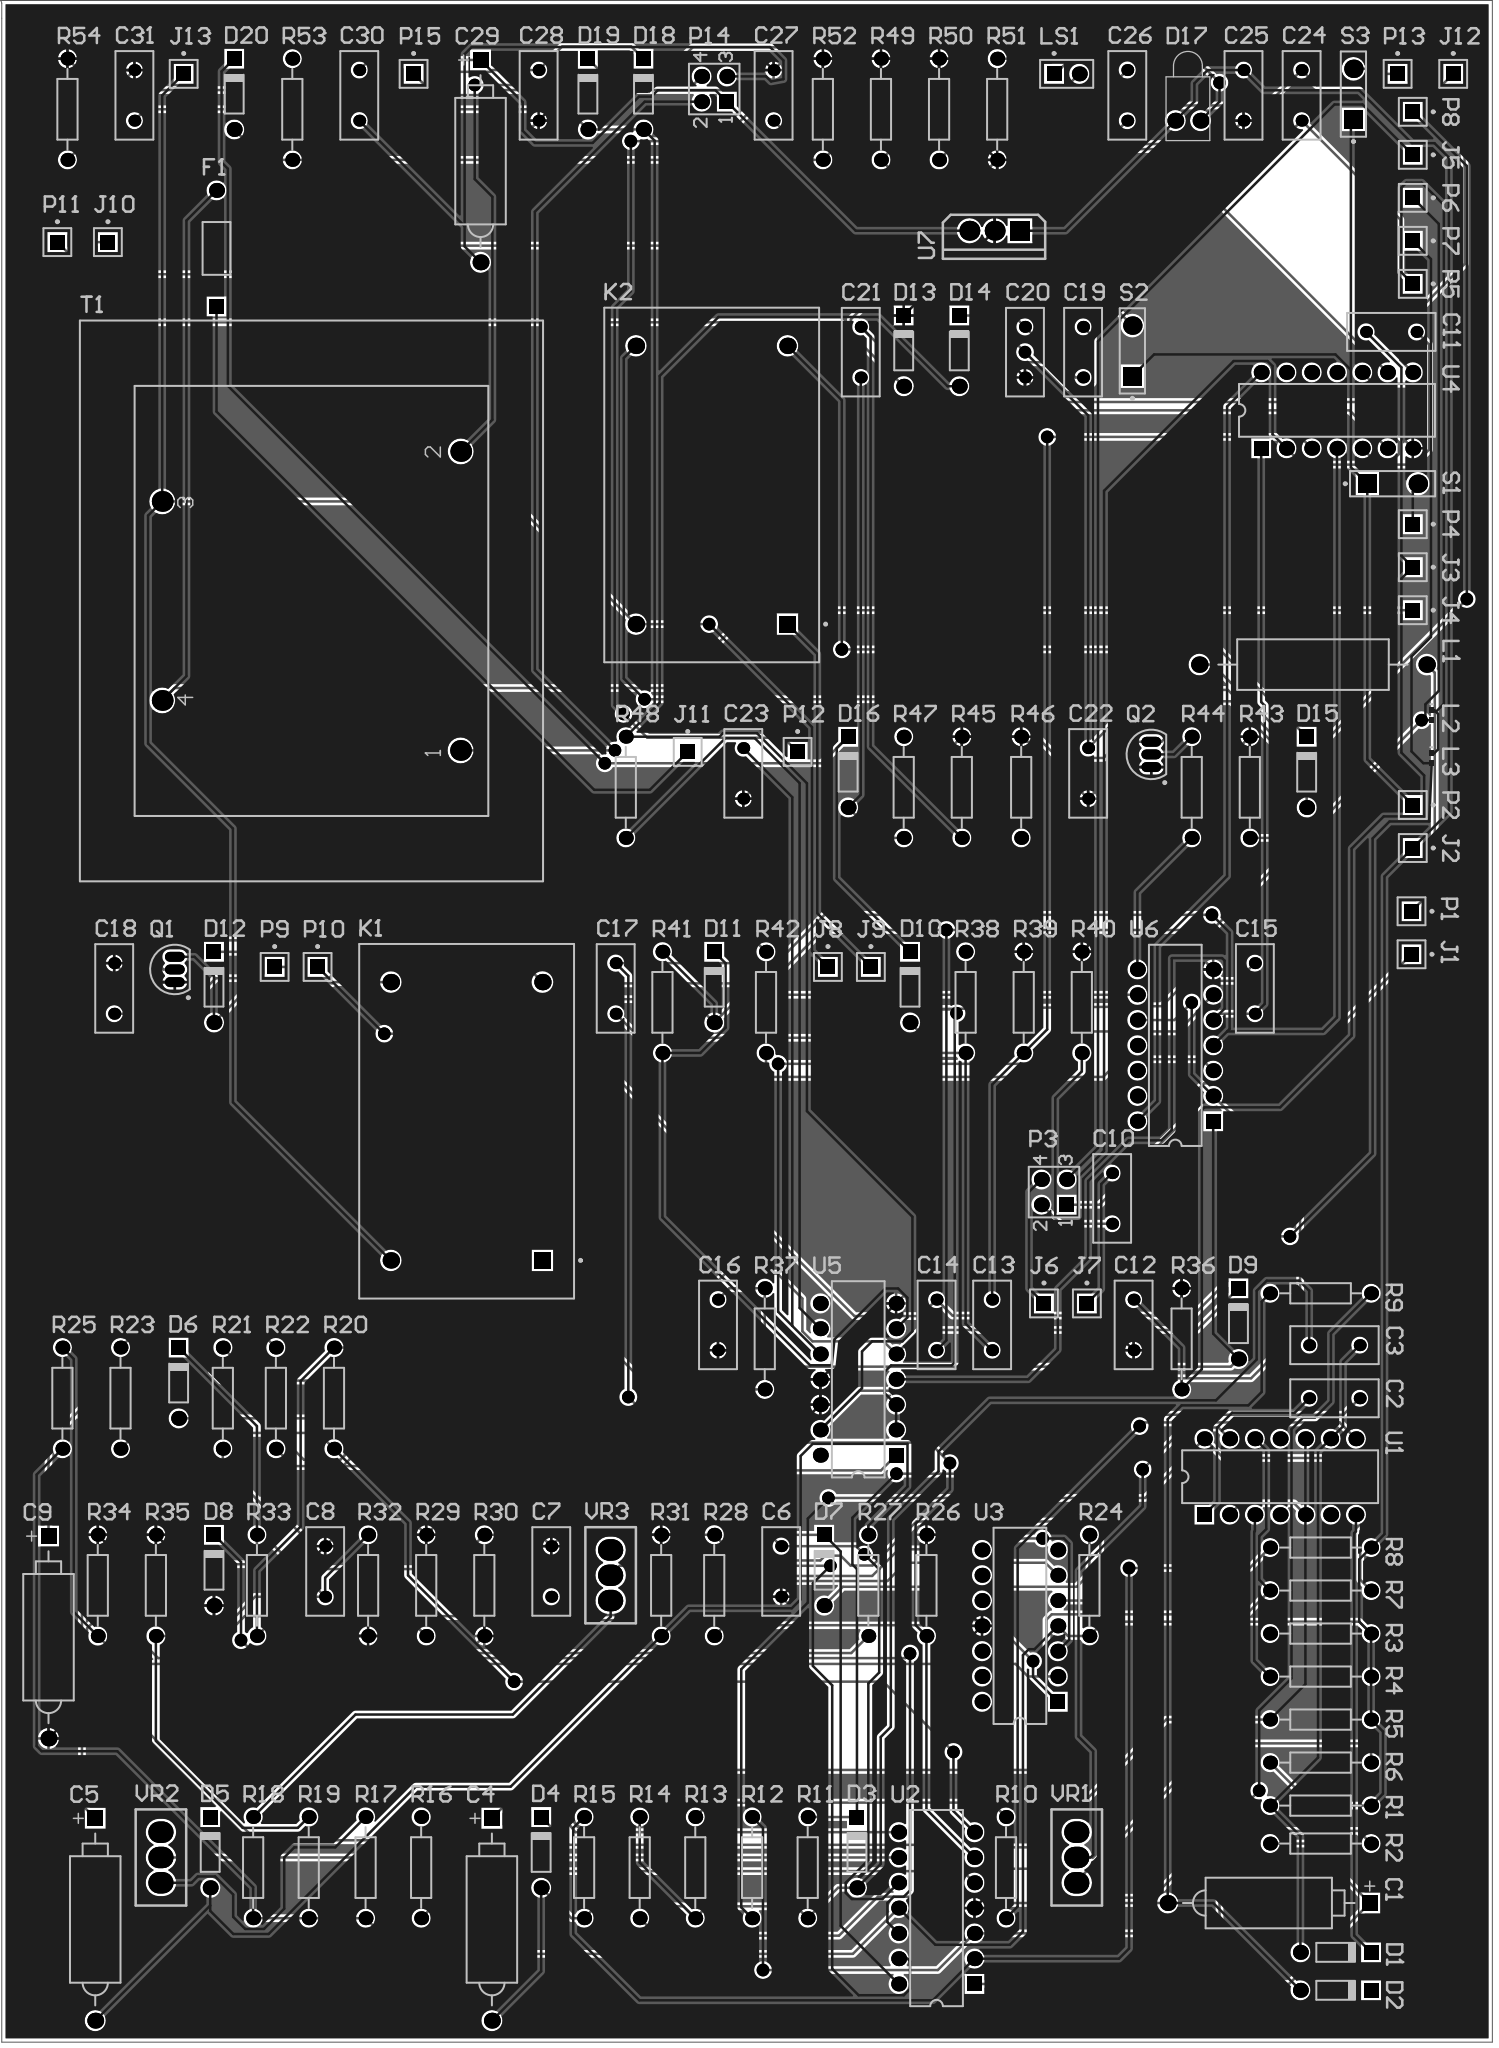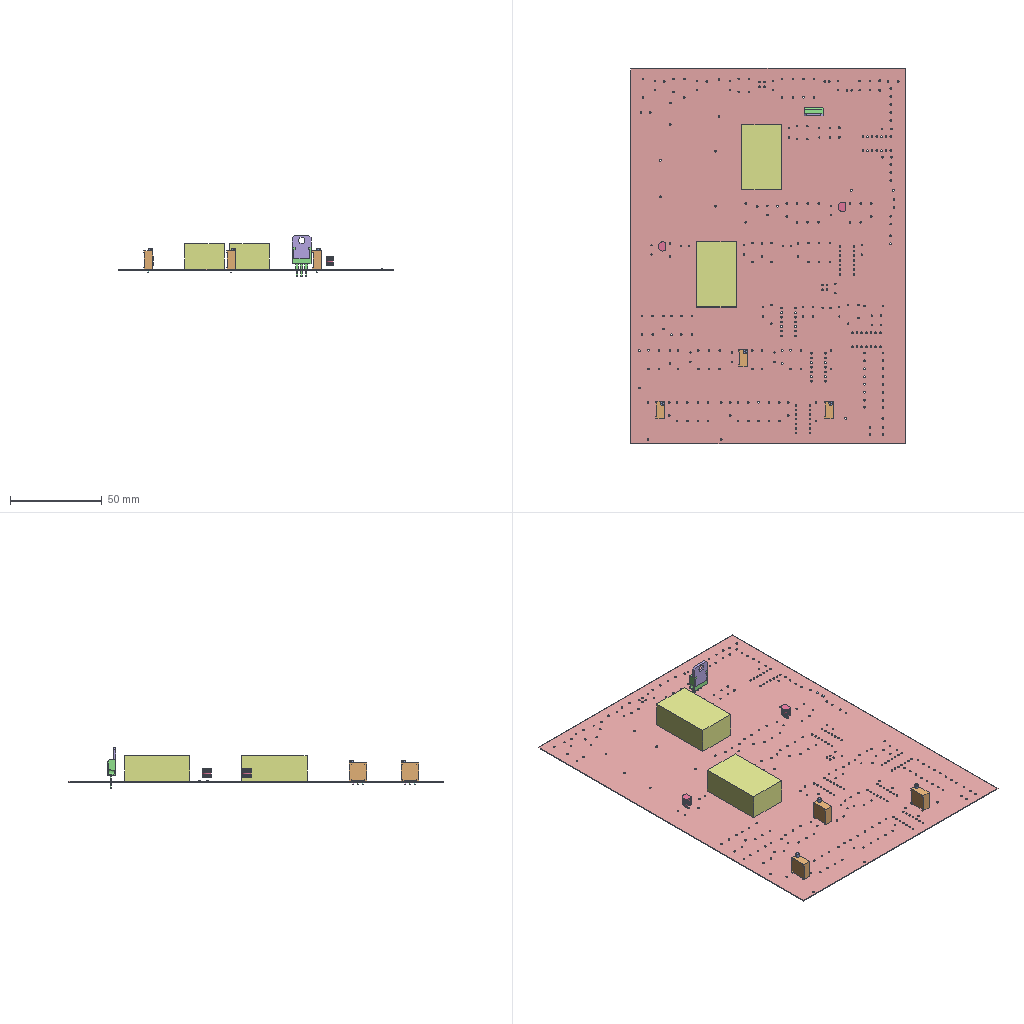Circuit board layout | Altium Designer | box 150 x 205 x 22.5 mm
Layer stack:
# Altium Designer layer stack of  (unit mm; dielectric type: 0 none, 1 core, 2 prepreg, 3 surface material)
index,name,kind,layer,copper_thickness_mm,dielectric_type,dielectric_thickness_mm,dielectric_material,dielectric_constant
0,Top Paste,other,,,,,,
1,Top Overlay,other,,,,,,
2,Top Solder,dielectric,,,3,0.0102,Solder Resist,3.5
3,Top Layer,copper,Top Layer,0.0356,,,,
4,Dielectric 1,dielectric,,,0,0.32,FR-4,4.8
5,Bottom Layer,copper,Bottom Layer,0.0356,,,,
6,Bottom Solder,dielectric,,,3,0.0102,Solder Resist,3.5
7,Bottom Overlay,other,,,,,,
8,Bottom Paste,other,,,,,,
# drill layer pairs: low layer,high layer
drill_pair,Top Layer,Bottom Layer
Part placement:
Designator,Comment,Layer,Footprint,Center-X(mm),Center-Y(mm),Rotation
VR3,10K,TopLayer,3296W,143.764,65.926,90
VR2,10K,TopLayer,3296W,98.552,37.592,90
VR1,10K,TopLayer,3296W,190.627,37.592,90
U7,LM7805,TopLayer,TO220A,182.372,200.914,180
U6,SN74LS08J,TopLayer,J014,200.533,119.126,90
U5,SN74LS74AN,TopLayer,646-06,168.656,85.598,90
U4,SN74LS02N,TopLayer,N014,216.789,182.88,360
U3,LM324N,TopLayer,646-06,184.912,60.846,90
U2,LM324N,TopLayer,646-06,176.53,32.512,90
U1,LM324N,TopLayer,646-06,211.074,75.819,360
T1,Trans Eq,TopLayer,TRF_4,113.686,163.745,90
S3,SW-PB,TopLayer,SPST-2,218.44,214.63,90
S2,SW-PB,TopLayer,SPST-2,196.215,188.849,90
S1,SW-PB,TopLayer,SPST-2,222.377,175.514,360
R54,51K,TopLayer,AXIAL-0.4,89.154,213.106,90
R53,51K,TopLayer,AXIAL-0.4,111.76,213.106,90
R52,51K,TopLayer,AXIAL-0.4,165.1,213.106,90
R51,15K,TopLayer,AXIAL-0.4,182.626,213.106,90
R50,51K,TopLayer,AXIAL-0.4,176.784,213.106,90
R49,51K,TopLayer,AXIAL-0.4,170.942,213.106,90
R48,10K,TopLayer,AXIAL-0.4,145.288,145.034,90
R47,5.1K,TopLayer,AXIAL-0.4,173.228,145.034,90
R46,5.1K,TopLayer,AXIAL-0.4,185.039,145.034,90
R45,5.1K,TopLayer,AXIAL-0.4,179.07,145.034,90
R44,1K,TopLayer,AXIAL-0.4,202.184,145.034,90
R43,51K,TopLayer,AXIAL-0.4,208.026,145.034,90
R42,1K,TopLayer,AXIAL-0.4,159.385,123.444,90
R41,510K,TopLayer,AXIAL-0.4,148.971,123.444,90
R40,5.1K,TopLayer,AXIAL-0.4,191.135,123.444,90
R39,5.1K,TopLayer,AXIAL-0.4,185.293,123.444,90
R38,5.1K,TopLayer,AXIAL-0.4,179.451,123.444,90
R37,510K,TopLayer,AXIAL-0.4,159.258,89.662,90
R36,49,TopLayer,AXIAL-0.4,201.168,89.662,90
R35,10K,TopLayer,AXIAL-0.4,98.044,64.91,90
R34,3M,TopLayer,AXIAL-0.4,92.202,64.91,90
R33,28,TopLayer,AXIAL-0.4,108.204,64.91,90
R32,10K,TopLayer,AXIAL-0.4,119.38,64.91,90
R31,25K,TopLayer,AXIAL-0.4,148.844,64.91,90
R30,100K,TopLayer,AXIAL-0.4,131.064,64.91,90
R29,35,TopLayer,AXIAL-0.4,125.222,64.91,90
R28,1K,TopLayer,AXIAL-0.4,154.178,64.91,90
R27,1K,TopLayer,AXIAL-0.4,169.672,64.91,90
R26,49,TopLayer,AXIAL-0.4,175.514,64.91,90
R25,10K,TopLayer,AXIAL-0.4,88.646,83.706,90
R24,10K,TopLayer,AXIAL-0.4,191.897,64.91,90
R23,50,TopLayer,AXIAL-0.4,94.488,83.706,90
R22,10K,TopLayer,AXIAL-0.4,110.109,83.706,90
R21,330K,TopLayer,AXIAL-0.4,104.775,83.706,90
R20,51,TopLayer,AXIAL-0.4,115.951,83.706,90
R19,10K,TopLayer,AXIAL-0.4,113.411,36.576,90
R18,10K,TopLayer,AXIAL-0.4,107.823,36.576,90
R17,50,TopLayer,AXIAL-0.4,119.126,36.576,90
R16,20K,TopLayer,AXIAL-0.4,124.714,36.576,90
R15,50,TopLayer,AXIAL-0.4,141.097,36.576,90
R14,2,TopLayer,AXIAL-0.4,146.685,36.576,90
R13,11,TopLayer,AXIAL-0.4,152.273,36.576,90
R12,22,TopLayer,AXIAL-0.4,157.988,36.576,90
R11,12,TopLayer,AXIAL-0.4,163.576,36.576,90
R10,1.5K,TopLayer,AXIAL-0.4,183.515,36.576,90
R9,24,TopLayer,AXIAL-0.4,215.138,94.234,360
R8,50,TopLayer,AXIAL-0.4,215.138,68.707,360
R7,50,TopLayer,AXIAL-0.4,215.138,64.389,360
R6,50,TopLayer,AXIAL-0.4,215.138,47.117,360
R5,10,TopLayer,AXIAL-0.4,215.138,51.435,360
R4,9,TopLayer,AXIAL-0.4,215.138,55.753,360
R3,8,TopLayer,AXIAL-0.4,215.138,60.071,360
R2,4,TopLayer,AXIAL-0.4,215.138,38.989,360
R1,17,TopLayer,AXIAL-0.4,215.138,42.799,360
Q2,2N3904,TopLayer,TO-92A,198.12,148.336,0
Q1,2N3904,TopLayer,TO-92A,99.949,126.746,0
P15,Plug,TopLayer,PIN1,123.952,216.662,0
P14,Header 2X2,TopLayer,HDR2X2,154.178,215.138,90
P13,Plug,TopLayer,PIN1,222.885,216.662,0
P12,Plug,TopLayer,PIN1,162.56,148.59,0
P11,Plug,TopLayer,PIN1,88.138,199.771,0
P10,Plug,TopLayer,PIN1,114.3,127,0
P9,Plug,TopLayer,PIN1,109.982,127,0
P8,Plug,TopLayer,PIN1,224.409,212.852,270
P7,Plug,TopLayer,PIN1,224.409,199.898,270
P6,Plug,TopLayer,PIN1,224.409,204.216,270
P5,Plug,TopLayer,PIN1,224.409,195.58,270
P4,Plug,TopLayer,PIN1,224.409,171.45,270
P3,Header 2X2,TopLayer,HDR2X2,188.341,104.394,90
P2,Plug,TopLayer,PIN1,224.409,143.256,270
P1,Plug,TopLayer,PIN1,224.282,132.588,270
LS1,Bell,TopLayer,PIN2,189.611,216.662,0
L3,Inductor,TopLayer,0402-A,226.314,147.955,270
L2,Inductor,TopLayer,0402-A,226.314,152.273,270
L1,Inductor Iron,TopLayer,AXIAL-0.9,214.376,157.353,360
K2,Relay-SPST,TopLayer,MODULE4,153.924,175.387,90
K1,Relay-SPST,TopLayer,MODULE4,129.286,111.506,90
J13,Socket,TopLayer,PIN1,100.838,216.662,0
J12,Socket,TopLayer,PIN1,228.473,216.662,0
J11,Socket,TopLayer,PIN1,151.511,148.59,0
J10,Socket,TopLayer,PIN1,93.218,199.771,0
J9,Socket,TopLayer,PIN1,169.926,127,0
J8,Socket,TopLayer,PIN1,165.608,127,0
J7,Socket,TopLayer,PIN1,191.643,93.218,0
J6,Socket,TopLayer,PIN1,187.325,93.218,0
J5,Socket,TopLayer,PIN1,224.409,208.534,270
J4,Socket,TopLayer,PIN1,224.409,162.814,270
J3,Socket,TopLayer,PIN1,224.409,167.132,270
J2,Socket,TopLayer,PIN1,224.409,138.938,270
J1,Socket,TopLayer,PIN1,224.282,128.27,270
F1,Fuse 1,TopLayer,PIN-W2/E2.8,104.14,199.136,90
D20,4148,TopLayer,DO-35,105.918,214.63,90
D19,4148,TopLayer,DO-35,141.478,214.63,90
D18,4148,TopLayer,DO-35,147.066,214.63,90
D17,LED1,TopLayer,LED-1,201.803,211.963,90
D16,4148,TopLayer,DO-35,167.64,146.558,90
D15,4148,TopLayer,DO-35,213.741,146.558,90
D14,4148,TopLayer,DO-35,178.816,188.849,90
D13,4148,TopLayer,DO-35,173.228,188.849,90
D12,4148,TopLayer,DO-35,103.886,124.968,90
D11,4148,TopLayer,DO-35,154.178,124.968,90
D10,4148,TopLayer,DO-35,173.863,124.968,90
D9,4148,TopLayer,DO-35,206.883,91.186,90
D8,4148,TopLayer,DO-35,103.886,66.434,90
D7,4148,TopLayer,DO-35,165.227,66.434,90
D6,4148,TopLayer,DO-35,100.33,85.23,90
D5,4148,TopLayer,DO-35,103.505,38.1,90
D4,4148,TopLayer,DO-35,136.779,38.1,90
D3,4148,TopLayer,DO-35,168.529,38.1,90
D2,4148,TopLayer,DO-35,216.662,24.257,360
D1,4148,TopLayer,DO-35,216.662,28.067,360
C31,105,TopLayer,RAD-0.2,95.885,214.503,90
C30,105,TopLayer,RAD-0.2,118.491,214.503,90
C29,220UF,TopLayer,POLAR0.8,130.683,207.899,90
C28,105,TopLayer,RAD-0.2,136.525,214.503,90
C27,105,TopLayer,RAD-0.2,160.147,214.503,90
C26,105,TopLayer,RAD-0.2,195.707,214.503,90
C25,105,TopLayer,RAD-0.2,207.391,214.503,90
C24,105,TopLayer,RAD-0.2,213.233,214.503,90
C23,104,TopLayer,RAD-0.2,157.099,146.431,90
C22,105,TopLayer,RAD-0.2,191.77,146.431,90
C21,104,TopLayer,RAD-0.2,168.91,188.722,90
C20,104,TopLayer,RAD-0.2,185.42,188.722,90
C19,104,TopLayer,RAD-0.2,191.262,188.722,90
C18,3.3U,TopLayer,RAD-0.2,93.853,124.841,90
C17,104,TopLayer,RAD-0.2,144.272,124.841,90
C16,3.3U,TopLayer,RAD-0.2,154.559,91.059,90
C15,104,TopLayer,RAD-0.2,208.534,124.841,90
C14,3.3U,TopLayer,RAD-0.2,176.53,91.059,90
C13,105,TopLayer,RAD-0.2,182.118,91.059,90
C12,105,TopLayer,RAD-0.2,196.342,91.059,90
C11,105,TopLayer,RAD-0.2,222.25,190.754,360
C10,3.3U,TopLayer,RAD-0.2,194.183,103.759,90
C9,220UF,TopLayer,POLAR0.8,87.249,59.703,90
C8,105,TopLayer,RAD-0.2,115.062,66.307,90
C7,105,TopLayer,RAD-0.2,137.795,66.307,90
C6,104,TopLayer,RAD-0.2,160.909,66.307,90
C5,10U,TopLayer,POLAR0.8,91.948,31.369,90
C4,220UF,TopLayer,POLAR0.8,131.826,31.369,90
C3,104,TopLayer,RAD-0.2,216.535,89.027,360
C2,0.002,TopLayer,RAD-0.2,216.535,83.693,360
C1,220UF,TopLayer,POLAR0.8,209.931,33.02,360
Pad and via stacks:
# Altium Designer via and pad stacks of  (unit mm). Each distinct definition once, with the count of objects using it.
# via: kind,start_layer,end_layer,hole_mm,diameter_mm,mode(0 simple;1 top-mid-bottom;2 full stack),diameter_per_layer,count,example_net
# pad: kind,layer,hole_mm,hole_type(0 round;1 square;2 slot),plating,top_size,top_shape(1 round;2 rect;3 octagon;9 rounded rect),mid_size,bottom_size,mode,footprint,size_per_layer,count,example
pad,Multi-Layer,0.9,0,plated,1.5x1.5,2,1.5x1.5,1.5x1.5,0,DO-35,,19,D2.2
pad,Multi-Layer,0.9,0,plated,1.5x1.5,1,1.5x1.5,1.5x1.5,0,DO-35,,19,D2.1
pad,Multi-Layer,1,0,plated,1.6x1.6,1,1.6x1.6,1.6x1.6,0,POLAR0.8,,5,C1.2
pad,Multi-Layer,1,0,plated,1.6x1.6,2,1.6x1.6,1.6x1.6,0,POLAR0.8,,5,C1.1
pad,Multi-Layer,0.85,0,plated,1.4x1.4,1,1.4x1.4,1.4x1.4,0,AXIAL-0.4,,108,R2.1
pad,Multi-Layer,0.9,0,plated,1.5x1.5,1,1.5x1.5,1.5x1.5,0,646-06,,52,U1.8
pad,Multi-Layer,0.9,0,plated,1.5x1.5,2,1.5x1.5,1.5x1.5,0,646-06,,4,U1.1
pad,Multi-Layer,0.7,0,plated,1.2x1.2,1,1.2x1.2,1.2x1.2,0,RAD-0.2,,52,C2.2
pad,Multi-Layer,0.889,0,plated,2.159x2.54,1,2.159x2.54,2.159x2.54,0,3296W,,9,VR1.3
pad,Multi-Layer,0.9,0,plated,1.5x1.5,2,1.5x1.5,1.5x1.5,0,PIN1,,26,J1.1
pad,Multi-Layer,0.9,0,plated,1.5x1.5,1,1.5x1.5,1.5x1.5,0,HDR2X2,,6,P3.4
pad,Multi-Layer,0.9,0,plated,1.5x1.5,2,1.5x1.5,1.5x1.5,0,HDR2X2,,2,P3.1
pad,Multi-Layer,1,0,plated,1.65x1.65,1,1.65x1.65,1.65x1.65,0,AXIAL-0.9,,2,L1.1
pad,Multi-Layer,1.1,0,plated,1.85x1.85,2,1.85x1.85,1.85x1.85,0,SPST-2,,3,S1.1
pad,Multi-Layer,1.1,0,plated,1.85x1.85,1,1.85x1.85,1.85x1.85,0,SPST-2,,3,S1.2
pad,Multi-Layer,0.9,0,plated,1.5x1.5,1,1.5x1.5,1.5x1.5,0,N014,,13,U4.8
pad,Multi-Layer,0.9,0,plated,1.5x1.5,2,1.5x1.5,1.5x1.5,0,N014,,1,U4.1
pad,Multi-Layer,0.9,0,plated,1.5x1.5,1,1.5x1.5,1.5x1.5,0,J014,,13,U6.8
pad,Multi-Layer,0.9,0,plated,1.5x1.5,2,1.5x1.5,1.5x1.5,0,J014,,1,U6.1
pad,Multi-Layer,1,0,plated,1.65x1.65,2,1.65x1.65,1.65x1.65,0,MODULE4,,2,K1.1
pad,Multi-Layer,1,0,plated,1.65x1.65,1,1.65x1.65,1.65x1.65,0,MODULE4,,6,K1.2
pad,Multi-Layer,0.9,0,plated,2x1,1,2x1,2x1,0,TO-92A,,6,Q1.3
pad,Multi-Layer,0.9,0,plated,1.5x1.5,1,1.5x1.5,1.5x1.5,0,PIN-W2/E2.8,,1,F1.2
pad,Multi-Layer,0.9,0,plated,1.5x1.5,2,1.5x1.5,1.5x1.5,0,PIN-W2/E2.8,,1,F1.1
pad,Multi-Layer,1.1,0,plated,2x2,1,2x2,2x2,0,TO220A,,2,U7.2
pad,Multi-Layer,1.1,0,plated,2x2,2,2x2,2x2,0,TO220A,,1,U7.1
pad,Multi-Layer,1.067,0,plated,2.083x2.083,1,2.083x2.083,2.083x2.083,0,TRF_4,,4,T1.1
pad,Multi-Layer,0.8,0,plated,1.6x1.6,1,1.6x1.6,1.6x1.6,0,LED-1,,2,D17.1
pad,Multi-Layer,0.9,0,plated,1.5x1.5,2,1.5x1.5,1.5x1.5,0,PIN2,,1,LS1.1
pad,Multi-Layer,0.9,0,plated,1.5x1.5,1,1.5x1.5,1.5x1.5,0,PIN2,,1,LS1.2
pad,Top Layer,0,0,plated,0.5x0.6,2,0.5x0.6,0.5x0.6,0,0402-A,,4,L3.2
via,Top Layer,Bottom Layer,0.7112,1.27,0,,37,NetC6_2
Copper pours:
name,layer,net,type(0 solid;1 hatched;2 none)
D,Top Layer,GND,0
D,Bottom Layer,GND,0
Design rules, without the lines most boards share:
# Altium Designer design rules of  (exported by Altium Designer, unit mm)
# columns: name | kind | enabled | priority | scope1 | scope2 | descriptor | typed fields (field=value)
SilkToSilkClearance | 55 | enabled | 1 | All | All | Silk to Silk (Clearance=0mil) (All),(All) |
SilkToSolderMaskClearance | 54 | enabled | 1 | IsPad | All | Silk To Solder Mask (Clearance=0mil) (IsPad),(All) |
MinimumSolderMaskSliver | 53 | enabled | 1 | All | All | Minimum Solder Mask Sliver (Gap=0mil) (All),(All) |
HoleToHoleClearance | 52 | enabled | 1 | All | All | Hole To Hole Clearance (Gap=10mil) (All),(All) | gap=0.254
DiffPairsRouting | 51 | enabled | 1 | All | All | Differential Pairs Uncoupled Length using the Gap Constraints (Min=10mil) (Max=10mil) (Prefered=10mil)  and Width Constraints (Min=15mil) (Max=15mil) (Prefered=15mil) (All) |
SolderMaskExpansion | 13 | enabled | 1 | All | All | Solder Mask Expansion (Expansion =4mil) (All) | expansion=0.1016
RoutingVias | 11 | enabled | 1 | All | All | Routing Via (MinHoleWidth=28mil) (MaxHoleWidth=28mil) (PreferredHoleWidth=28mil) (MinWidth=50mil) (MaxWidth=50mil) (PreferedWidth=50mil) (All) | via_min_hole=0.7112 via_max_hole=0.7112 via_preferred_diameter=1.27 via_preferred_hole=0.7112
Width | 2 | enabled | 1 | All | All | Width Constraint (Min=10mil) (Max=10mil) (Preferred=10mil) (All) |
PolygonConnect | 20 | enabled | 1 | All | All | Polygon Connect Rule(Relief Connect )(Conductor Width=10mil) (Relief Angle=90 Angle) (Entries=4) (Air Gap Width=10mil) (All),(All) | connect_style(0=relief,1=direct,2=none)=0 relief_conductor_width=0.254 relief_entries=4
PlaneConnect | 6 | enabled | 1 | All | All | Power Plane Connect Rule(Relief Connect )(Expansion=20mil) (Conductor Width=10mil) (Air Gap=10mil) (Entries=4) (All) | relief_conductor_width=0.254 relief_entries=4 relief_expansion=0.508
Clearance | 0 | enabled | 1 | All | All | Clearance Constraint (Gap=10mil) (All),(All) | gap=0.254
Classes set for this board:
# Altium Designer classes of  (member kind: 0 net, 1 component, 2 from-to, 3 pad, 4 layer, 5 differential pair, 6 design channel, 7 polygon, 8 structure, 9 xSignal)
# columns: class name | member kind | superclass | members
Sheet1 | 1 | no | C1; C2; C3; C4; C5; C6; C7; C8; C9; C10; C11; C12; C13; C14; C15; C16; C17; C18; C19; C20; C21; C22; C23; C24; C25; C26; C27; C28; C29; C30; C31; D1; D2; D3; D4; D5; D6; D7; D8; D9; D10; D11; D12; D13; D14; D15; D16; D17; D18; D19; D20; F1; J1; J2; J3; J4; J5; J6; J7; J8; J9; J10; J11; J12; J13; K1; K2; L1; L2; L3; LS1; P1; P2; P3; P4; P5; P6; P7; P8; P9; P10; P11; P12; P13; P14; P15; Q1; Q2; R1; R2; R3; R4; R5; R6; R7; R8; R9; R10; R11; R12; R13; R14; R15; R16; R17; R18; R19; R20; R21; R22; R23; R24; R25; R26; R27; R28; R29; R30; R31; R32; R33; R34; R35; R36; R37; R38; R39; R40; R41; R42; R43; R44; R45; R46; R47; R48; R49; R50; R51; R52; R53; R54; S1; S2; S3; T1; U1; U2; U3; U4; U5; U6; U7; VR1; VR2; VR3;